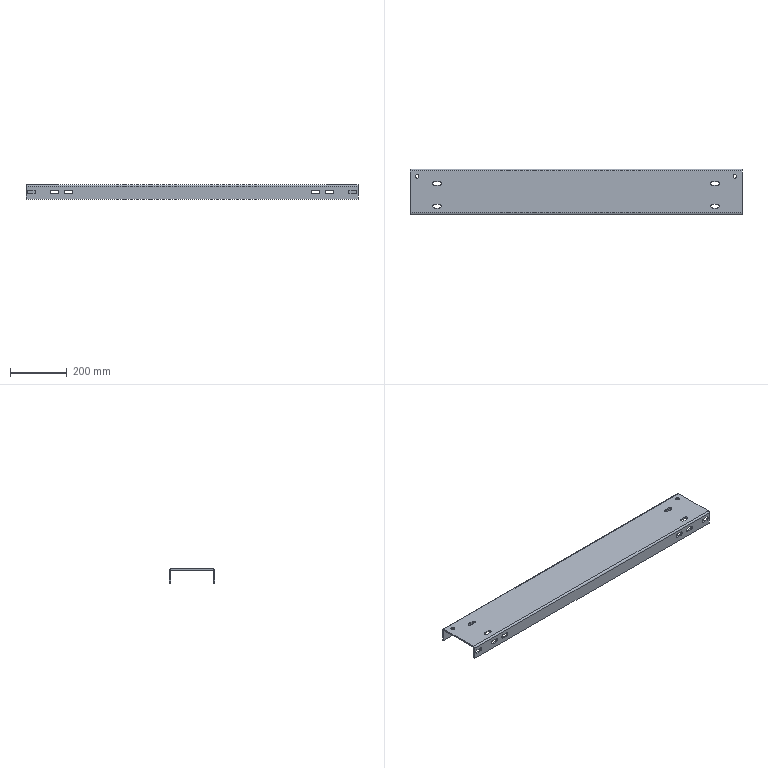Part | SolidWorks | features ICE 5, FlatPattern 1, SMBaseFlange 1, SheetMetal 1 | 1 solid | 86 faces | box 1170 x 160 x 50 mm | volume 1417867 mm3 | plane 46 | cylinder 40 | commonest cylinder face diameters 13 x20 14 x16 2 x2 12 x2